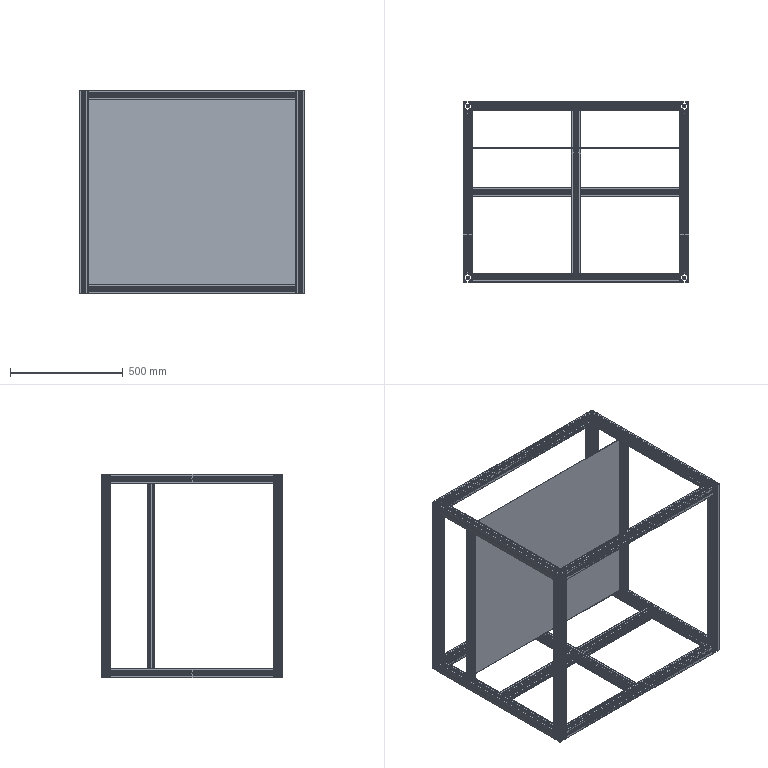Part | STEP file | Lower frame_aluminium extrusion<machined> | 18 solids | 2983 faces | box 1000 x 800 x 900 mm | volume 9363602 mm3 | cylinder 1555 | plane 1428 | commonest cylinder face diameters 1 x660 0.6 x557 4 x120 4.9 x120 6.8 x42 2 x32